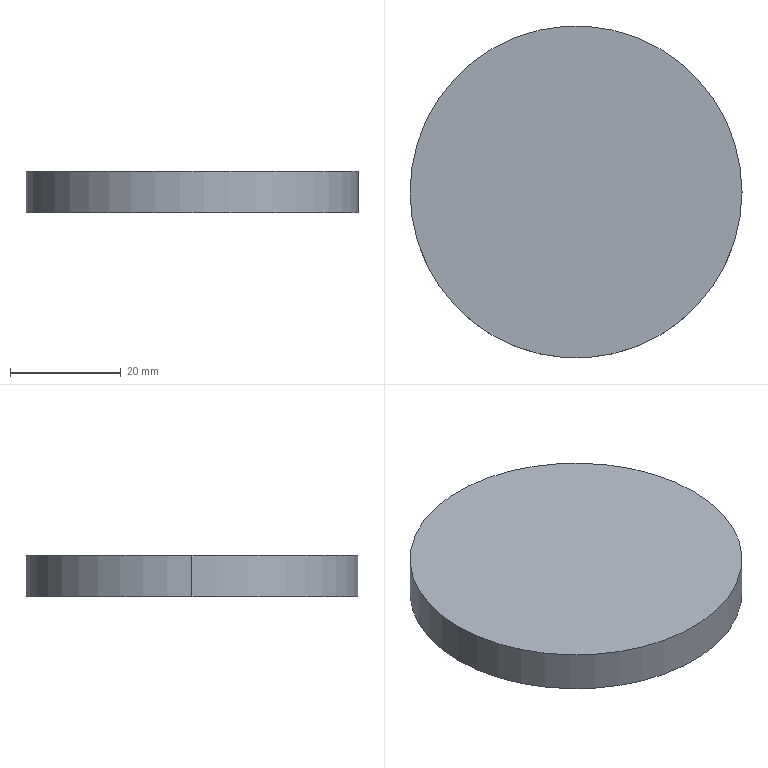Part | SolidWorks | features Extrusion 1 | 1 solid | 4 faces | box 60 x 60 x 7.5 mm | volume 21206 mm3 | cylinder 2 | plane 2 | commonest cylinder face diameters 60 x2
STEP:
#1=CARTESIAN_POINT('',(30.,0.,7.5));
#2=VERTEX_POINT('',#1);
#3=CARTESIAN_POINT('',(-30.,0.,7.5));
#4=VERTEX_POINT('',#3);
#5=CARTESIAN_POINT('',(0.,0.,7.5));
#6=DIRECTION('',(0.,0.,1.));
#7=DIRECTION('',(1.,0.,0.));
#8=AXIS2_PLACEMENT_3D('',#5,#6,#7);
#9=CIRCLE('',#8,30.);
#10=EDGE_CURVE('',#2,#4,#9,.T.);
#11=ORIENTED_EDGE('',*,*,#10,.F.);
#12=CARTESIAN_POINT('',(30.,0.,0.));
#13=VERTEX_POINT('',#12);
#14=CARTESIAN_POINT('',(30.,0.,7.5));
#15=DIRECTION('',(0.,0.,-1.));
#16=VECTOR('',#15,1000.);
#17=LINE('',#14,#16);
#18=EDGE_CURVE('',#2,#13,#17,.T.);
#19=ORIENTED_EDGE('',*,*,#18,.T.);
#20=CARTESIAN_POINT('',(-30.,0.,0.));
#21=VERTEX_POINT('',#20);
#22=CARTESIAN_POINT('',(0.,0.,0.));
#23=DIRECTION('',(0.,0.,1.));
#24=DIRECTION('',(1.,0.,0.));
#25=AXIS2_PLACEMENT_3D('',#22,#23,#24);
#26=CIRCLE('',#25,30.);
#27=EDGE_CURVE('',#13,#21,#26,.T.);
#28=ORIENTED_EDGE('',*,*,#27,.T.);
#29=CARTESIAN_POINT('',(-30.,0.,7.5));
#30=DIRECTION('',(0.,0.,-1.));
#31=VECTOR('',#30,1000.);
#32=LINE('',#29,#31);
#33=EDGE_CURVE('',#4,#21,#32,.T.);
#34=ORIENTED_EDGE('',*,*,#33,.F.);
#35=EDGE_LOOP('',(#11,#19,#28,#34));
#36=FACE_OUTER_BOUND('',#35,.T.);
#37=CARTESIAN_POINT('',(0.,0.,7.5));
#38=DIRECTION('',(0.,0.,-1.));
#39=DIRECTION('',(-1.,0.,0.));
#40=AXIS2_PLACEMENT_3D('',#37,#38,#39);
#41=CYLINDRICAL_SURFACE('',#40,30.);
#42=ADVANCED_FACE('',(#36),#41,.T.);
#43=ORIENTED_EDGE('',*,*,#18,.F.);
#44=CARTESIAN_POINT('',(0.,0.,7.5));
#45=DIRECTION('',(0.,0.,1.));
#46=DIRECTION('',(1.,0.,0.));
#47=AXIS2_PLACEMENT_3D('',#44,#45,#46);
#48=CIRCLE('',#47,30.);
#49=EDGE_CURVE('',#4,#2,#48,.T.);
#50=ORIENTED_EDGE('',*,*,#49,.F.);
#51=ORIENTED_EDGE('',*,*,#33,.T.);
#52=CARTESIAN_POINT('',(0.,0.,0.));
#53=DIRECTION('',(0.,0.,1.));
#54=DIRECTION('',(1.,0.,0.));
#55=AXIS2_PLACEMENT_3D('',#52,#53,#54);
#56=CIRCLE('',#55,30.);
#57=EDGE_CURVE('',#21,#13,#56,.T.);
#58=ORIENTED_EDGE('',*,*,#57,.T.);
#59=EDGE_LOOP('',(#43,#50,#51,#58));
#60=FACE_OUTER_BOUND('',#59,.T.);
#61=CARTESIAN_POINT('',(0.,0.,7.5));
#62=DIRECTION('',(0.,0.,-1.));
#63=DIRECTION('',(-1.,0.,0.));
#64=AXIS2_PLACEMENT_3D('',#61,#62,#63);
#65=CYLINDRICAL_SURFACE('',#64,30.);
#66=ADVANCED_FACE('',(#60),#65,.T.);
#67=ORIENTED_EDGE('',*,*,#49,.T.);
#68=ORIENTED_EDGE('',*,*,#10,.T.);
#69=EDGE_LOOP('',(#67,#68));
#70=FACE_OUTER_BOUND('',#69,.T.);
#71=CARTESIAN_POINT('',(0.,0.,7.5));
#72=DIRECTION('',(0.,0.,1.));
#73=DIRECTION('',(1.,0.,0.));
#74=AXIS2_PLACEMENT_3D('',#71,#72,#73);
#75=PLANE('',#74);
#76=ADVANCED_FACE('',(#70),#75,.T.);
#77=ORIENTED_EDGE('',*,*,#57,.F.);
#78=ORIENTED_EDGE('',*,*,#27,.F.);
#79=EDGE_LOOP('',(#77,#78));
#80=FACE_OUTER_BOUND('',#79,.T.);
#81=CARTESIAN_POINT('',(0.,0.,0.));
#82=DIRECTION('',(0.,0.,1.));
#83=DIRECTION('',(1.,0.,0.));
#84=AXIS2_PLACEMENT_3D('',#81,#82,#83);
#85=PLANE('',#84);
#86=ADVANCED_FACE('',(#80),#85,.F.);
#87=CLOSED_SHELL('',(#42,#66,#76,#86));
#88=MANIFOLD_SOLID_BREP('',#87);
#89=CARTESIAN_POINT('',(0.,0.,0.));
#90=DIRECTION('',(0.,0.,1.));
#91=DIRECTION('',(1.,0.,0.));
#92=AXIS2_PLACEMENT_3D('',#89,#90,#91);
#93=(LENGTH_UNIT()NAMED_UNIT(*)SI_UNIT(.MILLI.,.METRE.));
#94=UNCERTAINTY_MEASURE_WITH_UNIT(LENGTH_MEASURE(0.00001),#93,'','');
#95=(NAMED_UNIT(*)PLANE_ANGLE_UNIT()SI_UNIT($,.RADIAN.));
#96=(NAMED_UNIT(*)SI_UNIT($,.STERADIAN.)SOLID_ANGLE_UNIT());
#97=(GEOMETRIC_REPRESENTATION_CONTEXT(3)GLOBAL_UNCERTAINTY_ASSIGNED_CONTEXT((#94))GLOBAL_UNIT_ASSIGNED_CONTEXT((#93,#95,#96))REPRESENTATION_CONTEXT('',''));
#98=ADVANCED_BREP_SHAPE_REPRESENTATION('',(#88,#92),#97);